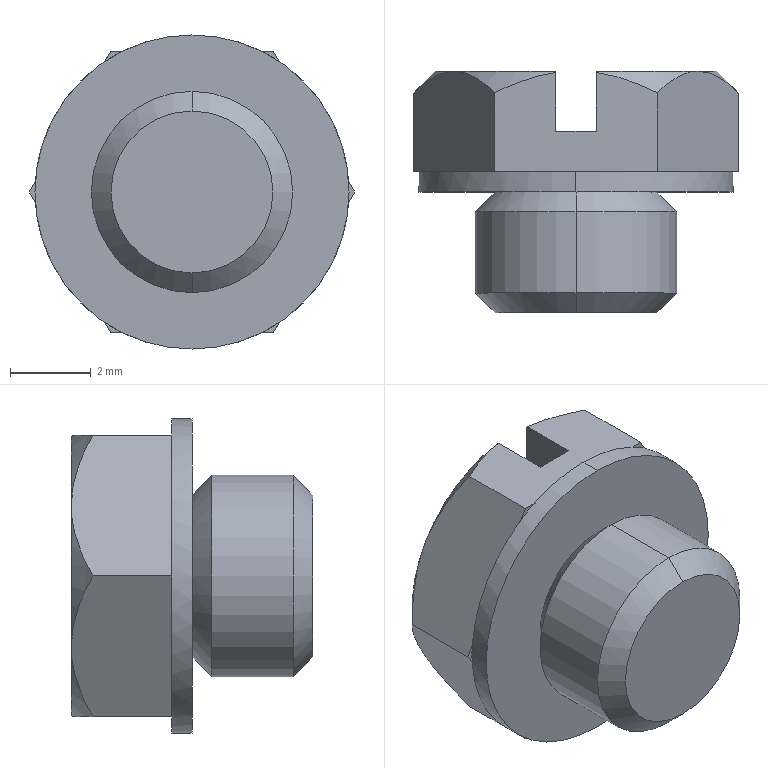Part | SolidWorks | features BaseBody 1 | 1 solid | 39 faces | box 8.083 x 6 x 7.8 mm | volume 174.211 mm3 | plane 25 | cone 10 | cylinder 4 | commonest cylinder face diameters 5 x2 7.8 x2
STEP:
#1=CARTESIAN_POINT('',(0.,-3.5,-2.01));
#2=VERTEX_POINT('',#1);
#3=CARTESIAN_POINT('',(0.,-3.5,2.01));
#4=VERTEX_POINT('',#3);
#5=CARTESIAN_POINT('',(0.,-3.5,0.));
#6=DIRECTION('',(0.,-1.,0.));
#7=DIRECTION('',(0.,0.,-1.));
#8=AXIS2_PLACEMENT_3D('',#5,#6,#7);
#9=CIRCLE('',#8,2.01);
#10=EDGE_CURVE('',#2,#4,#9,.T.);
#11=ORIENTED_EDGE('',*,*,#10,.F.);
#12=CARTESIAN_POINT('',(0.,-3.01,-2.5));
#13=VERTEX_POINT('',#12);
#14=CARTESIAN_POINT('',(0.,-3.01,-2.5));
#15=DIRECTION('',(0.,0.7071,-0.7071));
#16=VECTOR('',#15,1000.);
#17=LINE('',#14,#16);
#18=EDGE_CURVE('',#2,#13,#17,.T.);
#19=ORIENTED_EDGE('',*,*,#18,.T.);
#20=CARTESIAN_POINT('',(0.,-3.01,2.5));
#21=VERTEX_POINT('',#20);
#22=CARTESIAN_POINT('',(0.,-3.01,0.));
#23=DIRECTION('',(0.,-1.,0.));
#24=DIRECTION('',(0.,0.,-1.));
#25=AXIS2_PLACEMENT_3D('',#22,#23,#24);
#26=CIRCLE('',#25,2.5);
#27=EDGE_CURVE('',#13,#21,#26,.T.);
#28=ORIENTED_EDGE('',*,*,#27,.T.);
#29=CARTESIAN_POINT('',(0.,-3.01,2.5));
#30=DIRECTION('',(0.,0.7071,0.7071));
#31=VECTOR('',#30,1000.);
#32=LINE('',#29,#31);
#33=EDGE_CURVE('',#4,#21,#32,.T.);
#34=ORIENTED_EDGE('',*,*,#33,.F.);
#35=EDGE_LOOP('',(#11,#19,#28,#34));
#36=FACE_OUTER_BOUND('',#35,.T.);
#37=CARTESIAN_POINT('',(0.,-3.01,0.));
#38=DIRECTION('',(0.,1.,0.));
#39=DIRECTION('',(0.,0.,1.));
#40=AXIS2_PLACEMENT_3D('',#37,#38,#39);
#41=CONICAL_SURFACE('',#40,2.5,0.7854);
#42=ADVANCED_FACE('',(#36),#41,.T.);
#43=CARTESIAN_POINT('',(0.,-3.01,0.));
#44=DIRECTION('',(0.,-1.,0.));
#45=DIRECTION('',(0.,0.,-1.));
#46=AXIS2_PLACEMENT_3D('',#43,#44,#45);
#47=CIRCLE('',#46,2.5);
#48=EDGE_CURVE('',#21,#13,#47,.T.);
#49=ORIENTED_EDGE('',*,*,#48,.F.);
#50=CARTESIAN_POINT('',(0.,-0.9905,2.5));
#51=VERTEX_POINT('',#50);
#52=CARTESIAN_POINT('',(0.,-3.5,2.5));
#53=DIRECTION('',(0.,1.,0.));
#54=VECTOR('',#53,1000.);
#55=LINE('',#52,#54);
#56=EDGE_CURVE('',#21,#51,#55,.T.);
#57=ORIENTED_EDGE('',*,*,#56,.T.);
#58=CARTESIAN_POINT('',(0.,-0.9905,-2.5));
#59=VERTEX_POINT('',#58);
#60=CARTESIAN_POINT('',(0.,-0.9905,0.));
#61=DIRECTION('',(0.,-1.,0.));
#62=DIRECTION('',(0.,0.,-1.));
#63=AXIS2_PLACEMENT_3D('',#60,#61,#62);
#64=CIRCLE('',#63,2.5);
#65=EDGE_CURVE('',#51,#59,#64,.T.);
#66=ORIENTED_EDGE('',*,*,#65,.T.);
#67=CARTESIAN_POINT('',(0.,-3.5,-2.5));
#68=DIRECTION('',(0.,1.,0.));
#69=VECTOR('',#68,1000.);
#70=LINE('',#67,#69);
#71=EDGE_CURVE('',#13,#59,#70,.T.);
#72=ORIENTED_EDGE('',*,*,#71,.F.);
#73=EDGE_LOOP('',(#49,#57,#66,#72));
#74=FACE_OUTER_BOUND('',#73,.T.);
#75=CARTESIAN_POINT('',(0.,-3.5,0.));
#76=DIRECTION('',(0.,1.,0.));
#77=DIRECTION('',(0.,0.,-1.));
#78=AXIS2_PLACEMENT_3D('',#75,#76,#77);
#79=CYLINDRICAL_SURFACE('',#78,2.5);
#80=ADVANCED_FACE('',(#74),#79,.T.);
#81=CARTESIAN_POINT('',(0.,-0.5,-2.01));
#82=VERTEX_POINT('',#81);
#83=CARTESIAN_POINT('',(0.,-0.5,2.01));
#84=VERTEX_POINT('',#83);
#85=CARTESIAN_POINT('',(0.,-0.5,0.));
#86=DIRECTION('',(0.,-1.,0.));
#87=DIRECTION('',(0.,0.,-1.));
#88=AXIS2_PLACEMENT_3D('',#85,#86,#87);
#89=CIRCLE('',#88,2.01);
#90=EDGE_CURVE('',#82,#84,#89,.T.);
#91=ORIENTED_EDGE('',*,*,#90,.T.);
#92=CARTESIAN_POINT('',(0.,-0.5,2.01));
#93=DIRECTION('',(0.,-0.7071,0.7071));
#94=VECTOR('',#93,1000.);
#95=LINE('',#92,#94);
#96=EDGE_CURVE('',#84,#51,#95,.T.);
#97=ORIENTED_EDGE('',*,*,#96,.T.);
#98=CARTESIAN_POINT('',(0.,-0.9905,0.));
#99=DIRECTION('',(0.,-1.,0.));
#100=DIRECTION('',(0.,0.,-1.));
#101=AXIS2_PLACEMENT_3D('',#98,#99,#100);
#102=CIRCLE('',#101,2.5);
#103=EDGE_CURVE('',#59,#51,#102,.T.);
#104=ORIENTED_EDGE('',*,*,#103,.F.);
#105=CARTESIAN_POINT('',(0.,-0.5,-2.01));
#106=DIRECTION('',(0.,-0.7071,-0.7071));
#107=VECTOR('',#106,1000.);
#108=LINE('',#105,#107);
#109=EDGE_CURVE('',#82,#59,#108,.T.);
#110=ORIENTED_EDGE('',*,*,#109,.F.);
#111=EDGE_LOOP('',(#91,#97,#104,#110));
#112=FACE_OUTER_BOUND('',#111,.T.);
#113=CARTESIAN_POINT('',(0.,-0.5,0.));
#114=DIRECTION('',(0.,-1.,0.));
#115=DIRECTION('',(0.,0.,-1.));
#116=AXIS2_PLACEMENT_3D('',#113,#114,#115);
#117=CONICAL_SURFACE('',#116,2.01,0.7854);
#118=ADVANCED_FACE('',(#112),#117,.T.);
#119=CARTESIAN_POINT('',(0.,-0.5,3.9));
#120=VERTEX_POINT('',#119);
#121=CARTESIAN_POINT('',(0.,-0.5,-3.9));
#122=VERTEX_POINT('',#121);
#123=CARTESIAN_POINT('',(0.,-0.5,0.));
#124=DIRECTION('',(0.,-1.,0.));
#125=DIRECTION('',(0.,0.,-1.));
#126=AXIS2_PLACEMENT_3D('',#123,#124,#125);
#127=CIRCLE('',#126,3.9);
#128=EDGE_CURVE('',#120,#122,#127,.T.);
#129=ORIENTED_EDGE('',*,*,#128,.F.);
#130=CARTESIAN_POINT('',(0.,0.,3.9));
#131=VERTEX_POINT('',#130);
#132=CARTESIAN_POINT('',(0.,-0.5,3.9));
#133=DIRECTION('',(0.,1.,0.));
#134=VECTOR('',#133,1000.);
#135=LINE('',#132,#134);
#136=EDGE_CURVE('',#120,#131,#135,.T.);
#137=ORIENTED_EDGE('',*,*,#136,.T.);
#138=CARTESIAN_POINT('',(-1.72,0.,3.5));
#139=VERTEX_POINT('',#138);
#140=CARTESIAN_POINT('',(0.,0.,0.));
#141=DIRECTION('',(0.,-1.,0.));
#142=DIRECTION('',(0.,0.,-1.));
#143=AXIS2_PLACEMENT_3D('',#140,#141,#142);
#144=CIRCLE('',#143,3.9);
#145=EDGE_CURVE('',#131,#139,#144,.T.);
#146=ORIENTED_EDGE('',*,*,#145,.T.);
#147=CARTESIAN_POINT('',(-2.171,0.,3.24));
#148=VERTEX_POINT('',#147);
#149=CARTESIAN_POINT('',(0.,0.,0.));
#150=DIRECTION('',(0.,-1.,0.));
#151=DIRECTION('',(0.,0.,-1.));
#152=AXIS2_PLACEMENT_3D('',#149,#150,#151);
#153=CIRCLE('',#152,3.9);
#154=EDGE_CURVE('',#139,#148,#153,.T.);
#155=ORIENTED_EDGE('',*,*,#154,.T.);
#156=CARTESIAN_POINT('',(-3.891,0.,0.26));
#157=VERTEX_POINT('',#156);
#158=CARTESIAN_POINT('',(0.,0.,0.));
#159=DIRECTION('',(0.,-1.,0.));
#160=DIRECTION('',(0.,0.,-1.));
#161=AXIS2_PLACEMENT_3D('',#158,#159,#160);
#162=CIRCLE('',#161,3.9);
#163=EDGE_CURVE('',#148,#157,#162,.T.);
#164=ORIENTED_EDGE('',*,*,#163,.T.);
#165=CARTESIAN_POINT('',(-3.891,0.,-0.26));
#166=VERTEX_POINT('',#165);
#167=CARTESIAN_POINT('',(0.,0.,0.));
#168=DIRECTION('',(0.,-1.,0.));
#169=DIRECTION('',(0.,0.,-1.));
#170=AXIS2_PLACEMENT_3D('',#167,#168,#169);
#171=CIRCLE('',#170,3.9);
#172=EDGE_CURVE('',#157,#166,#171,.T.);
#173=ORIENTED_EDGE('',*,*,#172,.T.);
#174=CARTESIAN_POINT('',(-2.171,0.,-3.24));
#175=VERTEX_POINT('',#174);
#176=CARTESIAN_POINT('',(0.,0.,0.));
#177=DIRECTION('',(0.,-1.,0.));
#178=DIRECTION('',(0.,0.,-1.));
#179=AXIS2_PLACEMENT_3D('',#176,#177,#178);
#180=CIRCLE('',#179,3.9);
#181=EDGE_CURVE('',#166,#175,#180,.T.);
#182=ORIENTED_EDGE('',*,*,#181,.T.);
#183=CARTESIAN_POINT('',(-1.72,0.,-3.5));
#184=VERTEX_POINT('',#183);
#185=CARTESIAN_POINT('',(0.,0.,0.));
#186=DIRECTION('',(0.,-1.,0.));
#187=DIRECTION('',(0.,0.,-1.));
#188=AXIS2_PLACEMENT_3D('',#185,#186,#187);
#189=CIRCLE('',#188,3.9);
#190=EDGE_CURVE('',#175,#184,#189,.T.);
#191=ORIENTED_EDGE('',*,*,#190,.T.);
#192=CARTESIAN_POINT('',(0.,0.,-3.9));
#193=VERTEX_POINT('',#192);
#194=CARTESIAN_POINT('',(0.,0.,0.));
#195=DIRECTION('',(0.,-1.,0.));
#196=DIRECTION('',(0.,0.,-1.));
#197=AXIS2_PLACEMENT_3D('',#194,#195,#196);
#198=CIRCLE('',#197,3.9);
#199=EDGE_CURVE('',#184,#193,#198,.T.);
#200=ORIENTED_EDGE('',*,*,#199,.T.);
#201=CARTESIAN_POINT('',(0.,-0.5,-3.9));
#202=DIRECTION('',(0.,1.,0.));
#203=VECTOR('',#202,1000.);
#204=LINE('',#201,#203);
#205=EDGE_CURVE('',#122,#193,#204,.T.);
#206=ORIENTED_EDGE('',*,*,#205,.F.);
#207=EDGE_LOOP('',(#129,#137,#146,#155,#164,#173,#182,#191,#200,#206));
#208=FACE_OUTER_BOUND('',#207,.T.);
#209=CARTESIAN_POINT('',(0.,-0.5,0.));
#210=DIRECTION('',(0.,1.,0.));
#211=DIRECTION('',(0.,0.,-1.));
#212=AXIS2_PLACEMENT_3D('',#209,#210,#211);
#213=CYLINDRICAL_SURFACE('',#212,3.9);
#214=ADVANCED_FACE('',(#208),#213,.T.);
#215=CARTESIAN_POINT('',(-0.5,2.464,-3.5));
#216=VERTEX_POINT('',#215);
#217=CARTESIAN_POINT('',(-0.5,2.5,-3.464));
#218=VERTEX_POINT('',#217);
#219=CARTESIAN_POINT('',(-0.5,2.464,-3.5));
#220=CARTESIAN_POINT('',(-0.5,2.476,-3.488));
#221=CARTESIAN_POINT('',(-0.5,2.488,-3.476));
#222=CARTESIAN_POINT('',(-0.5,2.5,-3.464));
#223=B_SPLINE_CURVE_WITH_KNOTS('',3,(#219,#220,#221,#222),.UNSPECIFIED.,.F.,.F.,(4,4),(0.003913,0.003963),.UNSPECIFIED.);
#224=EDGE_CURVE('',#216,#218,#223,.T.);
#225=ORIENTED_EDGE('',*,*,#224,.F.);
#226=CARTESIAN_POINT('',(-2.021,1.959,-3.5));
#227=VERTEX_POINT('',#226);
#228=CARTESIAN_POINT('',(-0.5,2.464,-3.5));
#229=CARTESIAN_POINT('',(-0.6291,2.446,-3.5));
#230=CARTESIAN_POINT('',(-0.7576,2.421,-3.5));
#231=CARTESIAN_POINT('',(-0.9515,2.374,-3.5));
#232=CARTESIAN_POINT('',(-1.016,2.356,-3.5));
#233=CARTESIAN_POINT('',(-1.114,2.327,-3.5));
#234=CARTESIAN_POINT('',(-1.163,2.312,-3.5));
#235=CARTESIAN_POINT('',(-1.212,2.296,-3.5));
#236=CARTESIAN_POINT('',(-1.245,2.285,-3.5));
#237=CARTESIAN_POINT('',(-1.263,2.279,-3.5));
#238=CARTESIAN_POINT('',(-1.521,2.191,-3.5));
#239=CARTESIAN_POINT('',(-1.767,2.085,-3.5));
#240=CARTESIAN_POINT('',(-2.021,1.959,-3.5));
#241=B_SPLINE_CURVE_WITH_KNOTS('',3,(#228,#229,#230,#231,#232,#233,#234,#235,#236,#237,#238,#239,#240),.UNSPECIFIED.,.F.,.F.,(4,2,2,1,2,2,4),(0.,0.25,0.375,0.4375,0.4687,0.5,1.),.UNSPECIFIED.);
#242=EDGE_CURVE('',#216,#227,#241,.T.);
#243=ORIENTED_EDGE('',*,*,#242,.T.);
#244=CARTESIAN_POINT('',(-3.031,2.5,-1.75));
#245=VERTEX_POINT('',#244);
#246=CARTESIAN_POINT('',(-2.021,1.959,-3.5));
#247=CARTESIAN_POINT('',(-2.105,2.043,-3.354));
#248=CARTESIAN_POINT('',(-2.187,2.117,-3.212));
#249=CARTESIAN_POINT('',(-2.309,2.214,-3.001));
#250=CARTESIAN_POINT('',(-2.349,2.244,-2.932));
#251=CARTESIAN_POINT('',(-2.409,2.286,-2.827));
#252=CARTESIAN_POINT('',(-2.439,2.306,-2.775));
#253=CARTESIAN_POINT('',(-2.469,2.324,-2.723));
#254=CARTESIAN_POINT('',(-2.489,2.336,-2.689));
#255=CARTESIAN_POINT('',(-2.498,2.341,-2.673));
#256=CARTESIAN_POINT('',(-2.552,2.372,-2.58));
#257=CARTESIAN_POINT('',(-2.595,2.394,-2.505));
#258=CARTESIAN_POINT('',(-2.659,2.422,-2.394));
#259=CARTESIAN_POINT('',(-2.68,2.431,-2.358));
#260=CARTESIAN_POINT('',(-2.723,2.446,-2.284));
#261=CARTESIAN_POINT('',(-2.743,2.453,-2.248));
#262=CARTESIAN_POINT('',(-2.855,2.487,-2.056));
#263=CARTESIAN_POINT('',(-2.942,2.5,-1.904));
#264=CARTESIAN_POINT('',(-3.031,2.5,-1.75));
#265=B_SPLINE_CURVE_WITH_KNOTS('',3,(#246,#247,#248,#249,#250,#251,#252,#253,#254,#255,#256,#257,#258,#259,#260,#261,#262,#263,#264),.UNSPECIFIED.,.F.,.F.,(4,2,2,1,2,2,2,2,2,4),(0.,0.25,0.375,0.4375,0.4688,0.5,0.625,0.6875,0.75,1.),.UNSPECIFIED.);
#266=EDGE_CURVE('',#227,#245,#265,.T.);
#267=ORIENTED_EDGE('',*,*,#266,.T.);
#268=CARTESIAN_POINT('',(0.,2.5,0.));
#269=DIRECTION('',(0.,-1.,0.));
#270=DIRECTION('',(0.,0.,-1.));
#271=AXIS2_PLACEMENT_3D('',#268,#269,#270);
#272=CIRCLE('',#271,3.5);
#273=EDGE_CURVE('',#245,#218,#272,.T.);
#274=ORIENTED_EDGE('',*,*,#273,.T.);
#275=EDGE_LOOP('',(#225,#243,#267,#274));
#276=FACE_OUTER_BOUND('',#275,.T.);
#277=CARTESIAN_POINT('',(0.,2.5,0.));
#278=DIRECTION('',(0.,-1.,0.));
#279=DIRECTION('',(0.,0.,-1.));
#280=AXIS2_PLACEMENT_3D('',#277,#278,#279);
#281=CONICAL_SURFACE('',#280,3.5,0.7854);
#282=ADVANCED_FACE('',(#276),#281,.T.);
#283=CARTESIAN_POINT('',(-0.5,2.5,3.464));
#284=VERTEX_POINT('',#283);
#285=CARTESIAN_POINT('',(-0.5,2.464,3.5));
#286=VERTEX_POINT('',#285);
#287=CARTESIAN_POINT('',(-0.5,2.5,3.464));
#288=CARTESIAN_POINT('',(-0.5,2.488,3.476));
#289=CARTESIAN_POINT('',(-0.5,2.476,3.488));
#290=CARTESIAN_POINT('',(-0.5,2.464,3.5));
#291=B_SPLINE_CURVE_WITH_KNOTS('',3,(#287,#288,#289,#290),.UNSPECIFIED.,.F.,.F.,(4,4),(0.003847,0.003897),.UNSPECIFIED.);
#292=EDGE_CURVE('',#284,#286,#291,.T.);
#293=ORIENTED_EDGE('',*,*,#292,.T.);
#294=CARTESIAN_POINT('',(-0.5,1.,3.5));
#295=VERTEX_POINT('',#294);
#296=CARTESIAN_POINT('',(-0.5,5.,3.5));
#297=DIRECTION('',(0.,-1.,0.));
#298=VECTOR('',#297,1000.);
#299=LINE('',#296,#298);
#300=EDGE_CURVE('',#286,#295,#299,.T.);
#301=ORIENTED_EDGE('',*,*,#300,.T.);
#302=CARTESIAN_POINT('',(-0.5,1.,-3.5));
#303=VERTEX_POINT('',#302);
#304=CARTESIAN_POINT('',(-0.5,1.,5.));
#305=DIRECTION('',(0.,0.,-1.));
#306=VECTOR('',#305,1000.);
#307=LINE('',#304,#306);
#308=EDGE_CURVE('',#295,#303,#307,.T.);
#309=ORIENTED_EDGE('',*,*,#308,.T.);
#310=CARTESIAN_POINT('',(-0.5,5.,-3.5));
#311=DIRECTION('',(0.,1.,0.));
#312=VECTOR('',#311,1000.);
#313=LINE('',#310,#312);
#314=EDGE_CURVE('',#303,#216,#313,.T.);
#315=ORIENTED_EDGE('',*,*,#314,.T.);
#316=ORIENTED_EDGE('',*,*,#224,.T.);
#317=CARTESIAN_POINT('',(-0.5,2.5,5.));
#318=DIRECTION('',(0.,0.,-1.));
#319=VECTOR('',#318,1000.);
#320=LINE('',#317,#319);
#321=EDGE_CURVE('',#284,#218,#320,.T.);
#322=ORIENTED_EDGE('',*,*,#321,.F.);
#323=EDGE_LOOP('',(#293,#301,#309,#315,#316,#322));
#324=FACE_OUTER_BOUND('',#323,.T.);
#325=CARTESIAN_POINT('',(-0.5,2.5,5.));
#326=DIRECTION('',(1.,0.,0.));
#327=DIRECTION('',(0.,1.,0.));
#328=AXIS2_PLACEMENT_3D('',#325,#326,#327);
#329=PLANE('',#328);
#330=ADVANCED_FACE('',(#324),#329,.T.);
#331=CARTESIAN_POINT('',(2.171,0.,-3.24));
#332=VERTEX_POINT('',#331);
#333=CARTESIAN_POINT('',(3.891,0.,-0.26));
#334=VERTEX_POINT('',#333);
#335=CARTESIAN_POINT('',(0.,0.,0.));
#336=DIRECTION('',(0.,-1.,0.));
#337=DIRECTION('',(0.,0.,-1.));
#338=AXIS2_PLACEMENT_3D('',#335,#336,#337);
#339=CIRCLE('',#338,3.9);
#340=EDGE_CURVE('',#332,#334,#339,.T.);
#341=ORIENTED_EDGE('',*,*,#340,.F.);
#342=CARTESIAN_POINT('',(4.041,0.,0.));
#343=DIRECTION('',(0.5,0.,0.866));
#344=VECTOR('',#343,1000.);
#345=LINE('',#342,#344);
#346=EDGE_CURVE('',#332,#334,#345,.T.);
#347=ORIENTED_EDGE('',*,*,#346,.T.);
#348=EDGE_LOOP('',(#341,#347));
#349=FACE_OUTER_BOUND('',#348,.T.);
#350=CARTESIAN_POINT('',(0.,0.,0.));
#351=DIRECTION('',(0.,-1.,0.));
#352=DIRECTION('',(0.,0.,-1.));
#353=AXIS2_PLACEMENT_3D('',#350,#351,#352);
#354=PLANE('',#353);
#355=ADVANCED_FACE('',(#349),#354,.F.);
#356=CARTESIAN_POINT('',(3.891,0.,0.26));
#357=VERTEX_POINT('',#356);
#358=CARTESIAN_POINT('',(2.171,0.,3.24));
#359=VERTEX_POINT('',#358);
#360=CARTESIAN_POINT('',(0.,0.,0.));
#361=DIRECTION('',(0.,-1.,0.));
#362=DIRECTION('',(0.,0.,-1.));
#363=AXIS2_PLACEMENT_3D('',#360,#361,#362);
#364=CIRCLE('',#363,3.9);
#365=EDGE_CURVE('',#357,#359,#364,.T.);
#366=ORIENTED_EDGE('',*,*,#365,.F.);
#367=CARTESIAN_POINT('',(2.021,0.,3.5));
#368=DIRECTION('',(-0.5,0.,0.866));
#369=VECTOR('',#368,1000.);
#370=LINE('',#367,#369);
#371=EDGE_CURVE('',#357,#359,#370,.T.);
#372=ORIENTED_EDGE('',*,*,#371,.T.);
#373=EDGE_LOOP('',(#366,#372));
#374=FACE_OUTER_BOUND('',#373,.T.);
#375=CARTESIAN_POINT('',(0.,0.,0.));
#376=DIRECTION('',(0.,-1.,0.));
#377=DIRECTION('',(0.,0.,-1.));
#378=AXIS2_PLACEMENT_3D('',#375,#376,#377);
#379=PLANE('',#378);
#380=ADVANCED_FACE('',(#374),#379,.F.);
#381=ORIENTED_EDGE('',*,*,#199,.F.);
#382=CARTESIAN_POINT('',(1.72,0.,-3.5));
#383=VERTEX_POINT('',#382);
#384=CARTESIAN_POINT('',(2.021,0.,-3.5));
#385=DIRECTION('',(1.,0.,0.));
#386=VECTOR('',#385,1000.);
#387=LINE('',#384,#386);
#388=EDGE_CURVE('',#184,#383,#387,.T.);
#389=ORIENTED_EDGE('',*,*,#388,.T.);
#390=CARTESIAN_POINT('',(0.,0.,0.));
#391=DIRECTION('',(0.,-1.,0.));
#392=DIRECTION('',(0.,0.,-1.));
#393=AXIS2_PLACEMENT_3D('',#390,#391,#392);
#394=CIRCLE('',#393,3.9);
#395=EDGE_CURVE('',#193,#383,#394,.T.);
#396=ORIENTED_EDGE('',*,*,#395,.F.);
#397=EDGE_LOOP('',(#381,#389,#396));
#398=FACE_OUTER_BOUND('',#397,.T.);
#399=CARTESIAN_POINT('',(0.,0.,0.));
#400=DIRECTION('',(0.,-1.,0.));
#401=DIRECTION('',(0.,0.,-1.));
#402=AXIS2_PLACEMENT_3D('',#399,#400,#401);
#403=PLANE('',#402);
#404=ADVANCED_FACE('',(#398),#403,.F.);
#405=ORIENTED_EDGE('',*,*,#321,.T.);
#406=ORIENTED_EDGE('',*,*,#273,.F.);
#407=CARTESIAN_POINT('',(-3.031,2.5,1.75));
#408=VERTEX_POINT('',#407);
#409=CARTESIAN_POINT('',(0.,2.5,0.));
#410=DIRECTION('',(0.,-1.,0.));
#411=DIRECTION('',(0.,0.,-1.));
#412=AXIS2_PLACEMENT_3D('',#409,#410,#411);
#413=CIRCLE('',#412,3.5);
#414=EDGE_CURVE('',#408,#245,#413,.T.);
#415=ORIENTED_EDGE('',*,*,#414,.F.);
#416=CARTESIAN_POINT('',(0.,2.5,0.));
#417=DIRECTION('',(0.,-1.,0.));
#418=DIRECTION('',(0.,0.,-1.));
#419=AXIS2_PLACEMENT_3D('',#416,#417,#418);
#420=CIRCLE('',#419,3.5);
#421=EDGE_CURVE('',#284,#408,#420,.T.);
#422=ORIENTED_EDGE('',*,*,#421,.F.);
#423=EDGE_LOOP('',(#405,#406,#415,#422));
#424=FACE_OUTER_BOUND('',#423,.T.);
#425=CARTESIAN_POINT('',(0.,2.5,0.));
#426=DIRECTION('',(0.,-1.,0.));
#427=DIRECTION('',(0.,0.,-1.));
#428=AXIS2_PLACEMENT_3D('',#425,#426,#427);
#429=PLANE('',#428);
#430=ADVANCED_FACE('',(#424),#429,.F.);
#431=CARTESIAN_POINT('',(0.5,2.5,3.464));
#432=VERTEX_POINT('',#431);
#433=CARTESIAN_POINT('',(0.5,2.5,-3.464));
#434=VERTEX_POINT('',#433);
#435=CARTESIAN_POINT('',(0.5,2.5,5.));
#436=DIRECTION('',(0.,0.,-1.));
#437=VECTOR('',#436,1000.);
#438=LINE('',#435,#437);
#439=EDGE_CURVE('',#432,#434,#438,.T.);
#440=ORIENTED_EDGE('',*,*,#439,.F.);
#441=CARTESIAN_POINT('',(3.031,2.5,1.75));
#442=VERTEX_POINT('',#441);
#443=CARTESIAN_POINT('',(0.,2.5,0.));
#444=DIRECTION('',(0.,-1.,0.));
#445=DIRECTION('',(0.,0.,-1.));
#446=AXIS2_PLACEMENT_3D('',#443,#444,#445);
#447=CIRCLE('',#446,3.5);
#448=EDGE_CURVE('',#442,#432,#447,.T.);
#449=ORIENTED_EDGE('',*,*,#448,.F.);
#450=CARTESIAN_POINT('',(3.031,2.5,-1.75));
#451=VERTEX_POINT('',#450);
#452=CARTESIAN_POINT('',(0.,2.5,0.));
#453=DIRECTION('',(0.,-1.,0.));
#454=DIRECTION('',(0.,0.,-1.));
#455=AXIS2_PLACEMENT_3D('',#452,#453,#454);
#456=CIRCLE('',#455,3.5);
#457=EDGE_CURVE('',#451,#442,#456,.T.);
#458=ORIENTED_EDGE('',*,*,#457,.F.);
#459=CARTESIAN_POINT('',(0.,2.5,0.));
#460=DIRECTION('',(0.,-1.,0.));
#461=DIRECTION('',(0.,0.,-1.));
#462=AXIS2_PLACEMENT_3D('',#459,#460,#461);
#463=CIRCLE('',#462,3.5);
#464=EDGE_CURVE('',#434,#451,#463,.T.);
#465=ORIENTED_EDGE('',*,*,#464,.F.);
#466=EDGE_LOOP('',(#440,#449,#458,#465));
#467=FACE_OUTER_BOUND('',#466,.T.);
#468=CARTESIAN_POINT('',(0.,2.5,0.));
#469=DIRECTION('',(0.,-1.,0.));
#470=DIRECTION('',(0.,0.,-1.));
#471=AXIS2_PLACEMENT_3D('',#468,#469,#470);
#472=PLANE('',#471);
#473=ADVANCED_FACE('',(#467),#472,.F.);
#474=CARTESIAN_POINT('',(1.72,0.,3.5));
#475=VERTEX_POINT('',#474);
#476=CARTESIAN_POINT('',(0.,0.,0.));
#477=DIRECTION('',(0.,-1.,0.));
#478=DIRECTION('',(0.,0.,-1.));
#479=AXIS2_PLACEMENT_3D('',#476,#477,#478);
#480=CIRCLE('',#479,3.9);
#481=EDGE_CURVE('',#475,#131,#480,.T.);
#482=ORIENTED_EDGE('',*,*,#481,.F.);
#483=CARTESIAN_POINT('',(-2.021,0.,3.5));
#484=DIRECTION('',(-1.,0.,0.));
#485=VECTOR('',#484,1000.);
#486=LINE('',#483,#485);
#487=EDGE_CURVE('',#475,#139,#486,.T.);
#488=ORIENTED_EDGE('',*,*,#487,.T.);
#489=ORIENTED_EDGE('',*,*,#145,.F.);
#490=EDGE_LOOP('',(#482,#488,#489));
#491=FACE_OUTER_BOUND('',#490,.T.);
#492=CARTESIAN_POINT('',(0.,0.,0.));
#493=DIRECTION('',(0.,-1.,0.));
#494=DIRECTION('',(0.,0.,-1.));
#495=AXIS2_PLACEMENT_3D('',#492,#493,#494);
#496=PLANE('',#495);
#497=ADVANCED_FACE('',(#491),#496,.F.);
#498=ORIENTED_EDGE('',*,*,#163,.F.);
#499=CARTESIAN_POINT('',(-4.041,0.,0.));
#500=DIRECTION('',(0.5,0.,0.866));
#501=VECTOR('',#500,1000.);
#502=LINE('',#499,#501);
#503=EDGE_CURVE('',#157,#148,#502,.T.);
#504=ORIENTED_EDGE('',*,*,#503,.F.);
#505=EDGE_LOOP('',(#498,#504));
#506=FACE_OUTER_BOUND('',#505,.T.);
#507=CARTESIAN_POINT('',(0.,0.,0.));
#508=DIRECTION('',(0.,-1.,0.));
#509=DIRECTION('',(0.,0.,-1.));
#510=AXIS2_PLACEMENT_3D('',#507,#508,#509);
#511=PLANE('',#510);
#512=ADVANCED_FACE('',(#506),#511,.F.);
#513=ORIENTED_EDGE('',*,*,#136,.F.);
#514=CARTESIAN_POINT('',(0.,-0.5,0.));
#515=DIRECTION('',(0.,-1.,0.));
#516=DIRECTION('',(0.,0.,-1.));
#517=AXIS2_PLACEMENT_3D('',#514,#515,#516);
#518=CIRCLE('',#517,3.9);
#519=EDGE_CURVE('',#122,#120,#518,.T.);
#520=ORIENTED_EDGE('',*,*,#519,.F.);
#521=ORIENTED_EDGE('',*,*,#205,.T.);
#522=ORIENTED_EDGE('',*,*,#395,.T.);
#523=CARTESIAN_POINT('',(0.,0.,0.));
#524=DIRECTION('',(0.,-1.,0.));
#525=DIRECTION('',(0.,0.,-1.));
#526=AXIS2_PLACEMENT_3D('',#523,#524,#525);
#527=CIRCLE('',#526,3.9);
#528=EDGE_CURVE('',#383,#332,#527,.T.);
#529=ORIENTED_EDGE('',*,*,#528,.T.);
#530=ORIENTED_EDGE('',*,*,#340,.T.);
#531=CARTESIAN_POINT('',(0.,0.,0.));
#532=DIRECTION('',(0.,-1.,0.));
#533=DIRECTION('',(0.,0.,-1.));
#534=AXIS2_PLACEMENT_3D('',#531,#532,#533);
#535=CIRCLE('',#534,3.9);
#536=EDGE_CURVE('',#334,#357,#535,.T.);
#537=ORIENTED_EDGE('',*,*,#536,.T.);
#538=ORIENTED_EDGE('',*,*,#365,.T.);
#539=CARTESIAN_POINT('',(0.,0.,0.));
#540=DIRECTION('',(0.,-1.,0.));
#541=DIRECTION('',(0.,0.,-1.));
#542=AXIS2_PLACEMENT_3D('',#539,#540,#541);
#543=CIRCLE('',#542,3.9);
#544=EDGE_CURVE('',#359,#475,#543,.T.);
#545=ORIENTED_EDGE('',*,*,#544,.T.);
#546=ORIENTED_EDGE('',*,*,#481,.T.);
#547=EDGE_LOOP('',(#513,#520,#521,#522,#529,#530,#537,#538,#545,#546));
#548=FACE_OUTER_BOUND('',#547,.T.);
#549=CARTESIAN_POINT('',(0.,-0.5,0.));
#550=DIRECTION('',(0.,1.,0.));
#551=DIRECTION('',(0.,0.,-1.));
#552=AXIS2_PLACEMENT_3D('',#549,#550,#551);
#553=CYLINDRICAL_SURFACE('',#552,3.9);
#554=ADVANCED_FACE('',(#548),#553,.T.);
#555=ORIENTED_EDGE('',*,*,#181,.F.);
#556=CARTESIAN_POINT('',(-2.021,0.,-3.5));
#557=DIRECTION('',(0.5,0.,-0.866));
#558=VECTOR('',#557,1000.);
#559=LINE('',#556,#558);
#560=EDGE_CURVE('',#166,#175,#559,.T.);
#561=ORIENTED_EDGE('',*,*,#560,.T.);
#562=EDGE_LOOP('',(#555,#561));
#563=FACE_OUTER_BOUND('',#562,.T.);
#564=CARTESIAN_POINT('',(0.,0.,0.));
#565=DIRECTION('',(0.,-1.,0.));
#566=DIRECTION('',(0.,0.,-1.));
#567=AXIS2_PLACEMENT_3D('',#564,#565,#566);
#568=PLANE('',#567);
#569=ADVANCED_FACE('',(#563),#568,.F.);
#570=CARTESIAN_POINT('',(0.,-3.5,0.));
#571=DIRECTION('',(0.,-1.,0.));
#572=DIRECTION('',(0.,0.,-1.));
#573=AXIS2_PLACEMENT_3D('',#570,#571,#572);
#574=CIRCLE('',#573,2.01);
#575=EDGE_CURVE('',#4,#2,#574,.T.);
#576=ORIENTED_EDGE('',*,*,#575,.T.);
#577=ORIENTED_EDGE('',*,*,#10,.T.);
#578=EDGE_LOOP('',(#576,#577));
#579=FACE_OUTER_BOUND('',#578,.T.);
#580=CARTESIAN_POINT('',(2.01,-3.5,0.));
#581=DIRECTION('',(0.,1.,0.));
#582=DIRECTION('',(1.,0.,0.));
#583=AXIS2_PLACEMENT_3D('',#580,#581,#582);
#584=PLANE('',#583);
#585=ADVANCED_FACE('',(#579),#584,.F.);
#586=CARTESIAN_POINT('',(0.5,2.464,-3.5));
#587=VERTEX_POINT('',#586);
#588=CARTESIAN_POINT('',(0.5,2.5,-3.464));
#589=CARTESIAN_POINT('',(0.5,2.488,-3.476));
#590=CARTESIAN_POINT('',(0.5,2.476,-3.488));
#591=CARTESIAN_POINT('',(0.5,2.464,-3.5));
#592=B_SPLINE_CURVE_WITH_KNOTS('',3,(#588,#589,#590,#591),.UNSPECIFIED.,.F.,.F.,(4,4),(0.003823,0.003873),.UNSPECIFIED.);
#593=EDGE_CURVE('',#434,#587,#592,.T.);
#594=ORIENTED_EDGE('',*,*,#593,.F.);
#595=ORIENTED_EDGE('',*,*,#464,.T.);
#596=CARTESIAN_POINT('',(2.021,1.959,-3.5));
#597=VERTEX_POINT('',#596);
#598=CARTESIAN_POINT('',(3.031,2.5,-1.75));
#599=CARTESIAN_POINT('',(2.988,2.5,-1.825));
#600=CARTESIAN_POINT('',(2.944,2.497,-1.901));
#601=CARTESIAN_POINT('',(2.857,2.484,-2.051));
#602=CARTESIAN_POINT('',(2.813,2.474,-2.129));
#603=CARTESIAN_POINT('',(2.727,2.448,-2.277));
#604=CARTESIAN_POINT('',(2.684,2.433,-2.351));
#605=CARTESIAN_POINT('',(2.62,2.405,-2.462));
#606=CARTESIAN_POINT('',(2.588,2.39,-2.518));
#607=CARTESIAN_POINT('',(2.555,2.373,-2.574));
#608=CARTESIAN_POINT('',(2.534,2.362,-2.611));
#609=CARTESIAN_POINT('',(2.522,2.355,-2.631));
#610=CARTESIAN_POINT('',(2.352,2.258,-2.927));
#611=CARTESIAN_POINT('',(2.19,2.128,-3.207));
#612=CARTESIAN_POINT('',(2.021,1.959,-3.5));
#613=B_SPLINE_CURVE_WITH_KNOTS('',3,(#598,#599,#600,#601,#602,#603,#604,#605,#606,#607,#608,#609,#610,#611,#612),.UNSPECIFIED.,.F.,.F.,(4,2,2,2,1,2,2,4),(0.,0.125,0.25,0.375,0.4375,0.4687,0.5,1.),.UNSPECIFIED.);
#614=EDGE_CURVE('',#451,#597,#613,.T.);
#615=ORIENTED_EDGE('',*,*,#614,.T.);
#616=CARTESIAN_POINT('',(2.021,1.959,-3.5));
#617=CARTESIAN_POINT('',(1.894,2.022,-3.5));
#618=CARTESIAN_POINT('',(1.77,2.08,-3.5));
#619=CARTESIAN_POINT('',(1.585,2.158,-3.5));
#620=CARTESIAN_POINT('',(1.493,2.196,-3.5));
#621=CARTESIAN_POINT('',(1.386,2.236,-3.5));
#622=CARTESIAN_POINT('',(1.341,2.252,-3.5));
#623=CARTESIAN_POINT('',(1.31,2.263,-3.5));
#624=CARTESIAN_POINT('',(1.297,2.268,-3.5));
#625=CARTESIAN_POINT('',(1.016,2.364,-3.5));
#626=CARTESIAN_POINT('',(0.759,2.428,-3.5));
#627=CARTESIAN_POINT('',(0.5,2.464,-3.5));
#628=B_SPLINE_CURVE_WITH_KNOTS('',3,(#616,#617,#618,#619,#620,#621,#622,#623,#624,#625,#626,#627),.UNSPECIFIED.,.F.,.F.,(4,2,1,1,2,2,4),(0.,0.25,0.375,0.4375,0.4687,0.5,1.),.UNSPECIFIED.);
#629=EDGE_CURVE('',#597,#587,#628,.T.);
#630=ORIENTED_EDGE('',*,*,#629,.T.);
#631=EDGE_LOOP('',(#594,#595,#615,#630));
#632=FACE_OUTER_BOUND('',#631,.T.);
#633=CARTESIAN_POINT('',(0.,2.5,0.));
#634=DIRECTION('',(0.,-1.,0.));
#635=DIRECTION('',(0.,0.,-1.));
#636=AXIS2_PLACEMENT_3D('',#633,#634,#635);
#637=CONICAL_SURFACE('',#636,3.5,0.7854);
#638=ADVANCED_FACE('',(#632),#637,.T.);
#639=CARTESIAN_POINT('',(0.5,2.464,3.5));
#640=VERTEX_POINT('',#639);
#641=CARTESIAN_POINT('',(0.5,2.464,3.5));
#642=CARTESIAN_POINT('',(0.5,2.476,3.488));
#643=CARTESIAN_POINT('',(0.5,2.488,3.476));
#644=CARTESIAN_POINT('',(0.5,2.5,3.464));
#645=B_SPLINE_CURVE_WITH_KNOTS('',3,(#641,#642,#643,#644),.UNSPECIFIED.,.F.,.F.,(4,4),(0.003913,0.003963),.UNSPECIFIED.);
#646=EDGE_CURVE('',#640,#432,#645,.T.);
#647=ORIENTED_EDGE('',*,*,#646,.F.);
#648=CARTESIAN_POINT('',(2.021,1.959,3.5));
#649=VERTEX_POINT('',#648);
#650=CARTESIAN_POINT('',(0.5,2.464,3.5));
#651=CARTESIAN_POINT('',(0.6295,2.446,3.5));
#652=CARTESIAN_POINT('',(0.7583,2.421,3.5));
#653=CARTESIAN_POINT('',(0.9527,2.373,3.5));
#654=CARTESIAN_POINT('',(1.018,2.356,3.5));
#655=CARTESIAN_POINT('',(1.116,2.327,3.5));
#656=CARTESIAN_POINT('',(1.165,2.311,3.5));
#657=CARTESIAN_POINT('',(1.214,2.295,3.5));
#658=CARTESIAN_POINT('',(1.247,2.284,3.5));
#659=CARTESIAN_POINT('',(1.265,2.278,3.5));
#660=CARTESIAN_POINT('',(1.522,2.19,3.5));
#661=CARTESIAN_POINT('',(1.768,2.085,3.5));
#662=CARTESIAN_POINT('',(2.021,1.959,3.5));
#663=B_SPLINE_CURVE_WITH_KNOTS('',3,(#650,#651,#652,#653,#654,#655,#656,#657,#658,#659,#660,#661,#662),.UNSPECIFIED.,.F.,.F.,(4,2,2,1,2,2,4),(0.,0.25,0.375,0.4375,0.4687,0.5,1.),.UNSPECIFIED.);
#664=EDGE_CURVE('',#640,#649,#663,.T.);
#665=ORIENTED_EDGE('',*,*,#664,.T.);
#666=CARTESIAN_POINT('',(2.021,1.959,3.5));
#667=CARTESIAN_POINT('',(2.105,2.043,3.354));
#668=CARTESIAN_POINT('',(2.187,2.117,3.212));
#669=CARTESIAN_POINT('',(2.309,2.214,3.001));
#670=CARTESIAN_POINT('',(2.349,2.244,2.932));
#671=CARTESIAN_POINT('',(2.409,2.286,2.827));
#672=CARTESIAN_POINT('',(2.439,2.306,2.775));
#673=CARTESIAN_POINT('',(2.469,2.324,2.723));
#674=CARTESIAN_POINT('',(2.489,2.336,2.689));
#675=CARTESIAN_POINT('',(2.498,2.341,2.673));
#676=CARTESIAN_POINT('',(2.552,2.372,2.58));
#677=CARTESIAN_POINT('',(2.595,2.394,2.505));
#678=CARTESIAN_POINT('',(2.659,2.422,2.394));
#679=CARTESIAN_POINT('',(2.68,2.431,2.358));
#680=CARTESIAN_POINT('',(2.723,2.446,2.284));
#681=CARTESIAN_POINT('',(2.743,2.453,2.248));
#682=CARTESIAN_POINT('',(2.855,2.487,2.056));
#683=CARTESIAN_POINT('',(2.942,2.5,1.904));
#684=CARTESIAN_POINT('',(3.031,2.5,1.75));
#685=B_SPLINE_CURVE_WITH_KNOTS('',3,(#666,#667,#668,#669,#670,#671,#672,#673,#674,#675,#676,#677,#678,#679,#680,#681,#682,#683,#684),.UNSPECIFIED.,.F.,.F.,(4,2,2,1,2,2,2,2,2,4),(0.,0.25,0.375,0.4375,0.4687,0.5,0.625,0.6875,0.75,1.),.UNSPECIFIED.);
#686=EDGE_CURVE('',#649,#442,#685,.T.);
#687=ORIENTED_EDGE('',*,*,#686,.T.);
#688=ORIENTED_EDGE('',*,*,#448,.T.);
#689=EDGE_LOOP('',(#647,#665,#687,#688));
#690=FACE_OUTER_BOUND('',#689,.T.);
#691=CARTESIAN_POINT('',(0.,2.5,0.));
#692=DIRECTION('',(0.,-1.,0.));
#693=DIRECTION('',(0.,0.,-1.));
#694=AXIS2_PLACEMENT_3D('',#691,#692,#693);
#695=CONICAL_SURFACE('',#694,3.5,0.7854);
#696=ADVANCED_FACE('',(#690),#695,.T.);
#697=ORIENTED_EDGE('',*,*,#292,.F.);
#698=ORIENTED_EDGE('',*,*,#421,.T.);
#699=CARTESIAN_POINT('',(-2.021,1.959,3.5));
#700=VERTEX_POINT('',#699);
#701=CARTESIAN_POINT('',(-3.031,2.5,1.75));
#702=CARTESIAN_POINT('',(-2.988,2.5,1.825));
#703=CARTESIAN_POINT('',(-2.944,2.497,1.901));
#704=CARTESIAN_POINT('',(-2.857,2.484,2.051));
#705=CARTESIAN_POINT('',(-2.813,2.474,2.129));
#706=CARTESIAN_POINT('',(-2.727,2.448,2.277));
#707=CARTESIAN_POINT('',(-2.684,2.433,2.351));
#708=CARTESIAN_POINT('',(-2.62,2.405,2.462));
#709=CARTESIAN_POINT('',(-2.588,2.39,2.518));
#710=CARTESIAN_POINT('',(-2.555,2.373,2.574));
#711=CARTESIAN_POINT('',(-2.534,2.362,2.611));
#712=CARTESIAN_POINT('',(-2.522,2.355,2.631));
#713=CARTESIAN_POINT('',(-2.352,2.258,2.927));
#714=CARTESIAN_POINT('',(-2.19,2.128,3.207));
#715=CARTESIAN_POINT('',(-2.021,1.959,3.5));
#716=B_SPLINE_CURVE_WITH_KNOTS('',3,(#701,#702,#703,#704,#705,#706,#707,#708,#709,#710,#711,#712,#713,#714,#715),.UNSPECIFIED.,.F.,.F.,(4,2,2,2,1,2,2,4),(0.,0.125,0.25,0.375,0.4375,0.4687,0.5,1.),.UNSPECIFIED.);
#717=EDGE_CURVE('',#408,#700,#716,.T.);
#718=ORIENTED_EDGE('',*,*,#717,.T.);
#719=CARTESIAN_POINT('',(-2.021,1.959,3.5));
#720=CARTESIAN_POINT('',(-1.894,2.022,3.5));
#721=CARTESIAN_POINT('',(-1.769,2.08,3.5));
#722=CARTESIAN_POINT('',(-1.584,2.159,3.5));
#723=CARTESIAN_POINT('',(-1.491,2.196,3.5));
#724=CARTESIAN_POINT('',(-1.385,2.236,3.5));
#725=CARTESIAN_POINT('',(-1.339,2.253,3.5));
#726=CARTESIAN_POINT('',(-1.308,2.263,3.5));
#727=CARTESIAN_POINT('',(-1.295,2.268,3.5));
#728=CARTESIAN_POINT('',(-1.014,2.364,3.5));
#729=CARTESIAN_POINT('',(-0.7583,2.428,3.5));
#730=CARTESIAN_POINT('',(-0.5,2.464,3.5));
#731=B_SPLINE_CURVE_WITH_KNOTS('',3,(#719,#720,#721,#722,#723,#724,#725,#726,#727,#728,#729,#730),.UNSPECIFIED.,.F.,.F.,(4,2,1,1,2,2,4),(0.,0.25,0.375,0.4375,0.4688,0.5,1.),.UNSPECIFIED.);
#732=EDGE_CURVE('',#700,#286,#731,.T.);
#733=ORIENTED_EDGE('',*,*,#732,.T.);
#734=EDGE_LOOP('',(#697,#698,#718,#733));
#735=FACE_OUTER_BOUND('',#734,.T.);
#736=CARTESIAN_POINT('',(0.,2.5,0.));
#737=DIRECTION('',(0.,-1.,0.));
#738=DIRECTION('',(0.,0.,-1.));
#739=AXIS2_PLACEMENT_3D('',#736,#737,#738);
#740=CONICAL_SURFACE('',#739,3.5,0.7854);
#741=ADVANCED_FACE('',(#735),#740,.T.);
#742=ORIENTED_EDGE('',*,*,#300,.F.);
#743=ORIENTED_EDGE('',*,*,#732,.F.);
#744=CARTESIAN_POINT('',(-2.021,0.,3.5));
#745=VERTEX_POINT('',#744);
#746=CARTESIAN_POINT('',(-2.021,5.,3.5));
#747=DIRECTION('',(0.,-1.,0.));
#748=VECTOR('',#747,1000.);
#749=LINE('',#746,#748);
#750=EDGE_CURVE('',#700,#745,#749,.T.);
#751=ORIENTED_EDGE('',*,*,#750,.T.);
#752=CARTESIAN_POINT('',(-2.021,0.,3.5));
#753=DIRECTION('',(1.,0.,0.));
#754=VECTOR('',#753,1000.);
#755=LINE('',#752,#754);
#756=EDGE_CURVE('',#745,#139,#755,.T.);
#757=ORIENTED_EDGE('',*,*,#756,.T.);
#758=ORIENTED_EDGE('',*,*,#487,.F.);
#759=CARTESIAN_POINT('',(2.021,0.,3.5));
#760=VERTEX_POINT('',#759);
#761=CARTESIAN_POINT('',(-2.021,0.,3.5));
#762=DIRECTION('',(1.,0.,0.));
#763=VECTOR('',#762,1000.);
#764=LINE('',#761,#763);
#765=EDGE_CURVE('',#475,#760,#764,.T.);
#766=ORIENTED_EDGE('',*,*,#765,.T.);
#767=CARTESIAN_POINT('',(2.021,5.,3.5));
#768=DIRECTION('',(0.,-1.,0.));
#769=VECTOR('',#768,1000.);
#770=LINE('',#767,#769);
#771=EDGE_CURVE('',#649,#760,#770,.T.);
#772=ORIENTED_EDGE('',*,*,#771,.F.);
#773=ORIENTED_EDGE('',*,*,#664,.F.);
#774=CARTESIAN_POINT('',(0.5,1.,3.5));
#775=VERTEX_POINT('',#774);
#776=CARTESIAN_POINT('',(0.5,5.,3.5));
#777=DIRECTION('',(0.,1.,0.));
#778=VECTOR('',#777,1000.);
#779=LINE('',#776,#778);
#780=EDGE_CURVE('',#775,#640,#779,.T.);
#781=ORIENTED_EDGE('',*,*,#780,.F.);
#782=CARTESIAN_POINT('',(-2.021,1.,3.5));
#783=DIRECTION('',(1.,0.,0.));
#784=VECTOR('',#783,1000.);
#785=LINE('',#782,#784);
#786=EDGE_CURVE('',#295,#775,#785,.T.);
#787=ORIENTED_EDGE('',*,*,#786,.F.);
#788=EDGE_LOOP('',(#742,#743,#751,#757,#758,#766,#772,#773,#781,#787));
#789=FACE_OUTER_BOUND('',#788,.T.);
#790=CARTESIAN_POINT('',(-2.021,5.,3.5));
#791=DIRECTION('',(0.,0.,-1.));
#792=DIRECTION('',(0.,-1.,0.));
#793=AXIS2_PLACEMENT_3D('',#790,#791,#792);
#794=PLANE('',#793);
#795=ADVANCED_FACE('',(#789),#794,.F.);
#796=ORIENTED_EDGE('',*,*,#457,.T.);
#797=CARTESIAN_POINT('',(4.041,1.959,0.));
#798=VERTEX_POINT('',#797);
#799=CARTESIAN_POINT('',(3.031,2.5,1.75));
#800=CARTESIAN_POINT('',(3.075,2.5,1.675));
#801=CARTESIAN_POINT('',(3.118,2.497,1.599));
#802=CARTESIAN_POINT('',(3.205,2.484,1.449));
#803=CARTESIAN_POINT('',(3.25,2.474,1.371));
#804=CARTESIAN_POINT('',(3.335,2.448,1.223));
#805=CARTESIAN_POINT('',(3.378,2.433,1.149));
#806=CARTESIAN_POINT('',(3.442,2.405,1.038));
#807=CARTESIAN_POINT('',(3.475,2.39,0.982));
#808=CARTESIAN_POINT('',(3.507,2.373,0.926));
#809=CARTESIAN_POINT('',(3.528,2.362,0.8887));
#810=CARTESIAN_POINT('',(3.54,2.355,0.8687));
#811=CARTESIAN_POINT('',(3.711,2.258,0.5731));
#812=CARTESIAN_POINT('',(3.872,2.128,0.2932));
#813=CARTESIAN_POINT('',(4.041,1.959,0.));
#814=B_SPLINE_CURVE_WITH_KNOTS('',3,(#799,#800,#801,#802,#803,#804,#805,#806,#807,#808,#809,#810,#811,#812,#813),.UNSPECIFIED.,.F.,.F.,(4,2,2,2,1,2,2,4),(0.,0.125,0.25,0.375,0.4375,0.4688,0.5,1.),.UNSPECIFIED.);
#815=EDGE_CURVE('',#442,#798,#814,.T.);
#816=ORIENTED_EDGE('',*,*,#815,.T.);
#817=CARTESIAN_POINT('',(4.041,1.959,0.));
#818=CARTESIAN_POINT('',(3.957,2.043,-0.1456));
#819=CARTESIAN_POINT('',(3.875,2.117,-0.2879));
#820=CARTESIAN_POINT('',(3.753,2.214,-0.4987));
#821=CARTESIAN_POINT('',(3.713,2.244,-0.5684));
#822=CARTESIAN_POINT('',(3.653,2.286,-0.6727));
#823=CARTESIAN_POINT('',(3.623,2.306,-0.7247));
#824=CARTESIAN_POINT('',(3.593,2.324,-0.7766));
#825=CARTESIAN_POINT('',(3.573,2.336,-0.8111));
#826=CARTESIAN_POINT('',(3.564,2.341,-0.827));
#827=CARTESIAN_POINT('',(3.51,2.372,-0.9204));
#828=CARTESIAN_POINT('',(3.467,2.394,-0.9946));
#829=CARTESIAN_POINT('',(3.403,2.422,-1.106));
#830=CARTESIAN_POINT('',(3.382,2.431,-1.142));
#831=CARTESIAN_POINT('',(3.339,2.446,-1.216));
#832=CARTESIAN_POINT('',(3.319,2.453,-1.252));
#833=CARTESIAN_POINT('',(3.208,2.487,-1.444));
#834=CARTESIAN_POINT('',(3.12,2.5,-1.596));
#835=CARTESIAN_POINT('',(3.031,2.5,-1.75));
#836=B_SPLINE_CURVE_WITH_KNOTS('',3,(#817,#818,#819,#820,#821,#822,#823,#824,#825,#826,#827,#828,#829,#830,#831,#832,#833,#834,#835),.UNSPECIFIED.,.F.,.F.,(4,2,2,1,2,2,2,2,2,4),(0.,0.25,0.375,0.4375,0.4687,0.5,0.625,0.6875,0.75,1.),.UNSPECIFIED.);
#837=EDGE_CURVE('',#798,#451,#836,.T.);
#838=ORIENTED_EDGE('',*,*,#837,.T.);
#839=EDGE_LOOP('',(#796,#816,#838));
#840=FACE_OUTER_BOUND('',#839,.T.);
#841=CARTESIAN_POINT('',(0.,2.5,0.));
#842=DIRECTION('',(0.,-1.,0.));
#843=DIRECTION('',(0.,0.,-1.));
#844=AXIS2_PLACEMENT_3D('',#841,#842,#843);
#845=CONICAL_SURFACE('',#844,3.5,0.7854);
#846=ADVANCED_FACE('',(#840),#845,.T.);
#847=ORIENTED_EDGE('',*,*,#414,.T.);
#848=CARTESIAN_POINT('',(-4.041,1.959,0.));
#849=VERTEX_POINT('',#848);
#850=CARTESIAN_POINT('',(-3.031,2.5,-1.75));
#851=CARTESIAN_POINT('',(-3.075,2.5,-1.675));
#852=CARTESIAN_POINT('',(-3.118,2.497,-1.599));
#853=CARTESIAN_POINT('',(-3.205,2.484,-1.449));
#854=CARTESIAN_POINT('',(-3.25,2.474,-1.371));
#855=CARTESIAN_POINT('',(-3.335,2.448,-1.223));
#856=CARTESIAN_POINT('',(-3.378,2.433,-1.149));
#857=CARTESIAN_POINT('',(-3.442,2.405,-1.038));
#858=CARTESIAN_POINT('',(-3.475,2.39,-0.982));
#859=CARTESIAN_POINT('',(-3.507,2.373,-0.926));
#860=CARTESIAN_POINT('',(-3.528,2.362,-0.8887));
#861=CARTESIAN_POINT('',(-3.54,2.355,-0.8687));
#862=CARTESIAN_POINT('',(-3.711,2.258,-0.5731));
#863=CARTESIAN_POINT('',(-3.872,2.128,-0.2932));
#864=CARTESIAN_POINT('',(-4.041,1.959,0.));
#865=B_SPLINE_CURVE_WITH_KNOTS('',3,(#850,#851,#852,#853,#854,#855,#856,#857,#858,#859,#860,#861,#862,#863,#864),.UNSPECIFIED.,.F.,.F.,(4,2,2,2,1,2,2,4),(0.,0.125,0.25,0.375,0.4375,0.4687,0.5,1.),.UNSPECIFIED.);
#866=EDGE_CURVE('',#245,#849,#865,.T.);
#867=ORIENTED_EDGE('',*,*,#866,.T.);
#868=CARTESIAN_POINT('',(-4.041,1.959,0.));
#869=CARTESIAN_POINT('',(-3.957,2.043,0.1456));
#870=CARTESIAN_POINT('',(-3.875,2.117,0.2879));
#871=CARTESIAN_POINT('',(-3.753,2.214,0.4987));
#872=CARTESIAN_POINT('',(-3.713,2.244,0.5684));
#873=CARTESIAN_POINT('',(-3.653,2.286,0.6727));
#874=CARTESIAN_POINT('',(-3.623,2.306,0.7247));
#875=CARTESIAN_POINT('',(-3.593,2.324,0.7766));
#876=CARTESIAN_POINT('',(-3.573,2.336,0.8111));
#877=CARTESIAN_POINT('',(-3.564,2.341,0.827));
#878=CARTESIAN_POINT('',(-3.51,2.372,0.9204));
#879=CARTESIAN_POINT('',(-3.467,2.394,0.9946));
#880=CARTESIAN_POINT('',(-3.403,2.422,1.106));
#881=CARTESIAN_POINT('',(-3.382,2.431,1.142));
#882=CARTESIAN_POINT('',(-3.339,2.446,1.216));
#883=CARTESIAN_POINT('',(-3.319,2.453,1.252));
#884=CARTESIAN_POINT('',(-3.208,2.487,1.444));
#885=CARTESIAN_POINT('',(-3.12,2.5,1.596));
#886=CARTESIAN_POINT('',(-3.031,2.5,1.75));
#887=B_SPLINE_CURVE_WITH_KNOTS('',3,(#868,#869,#870,#871,#872,#873,#874,#875,#876,#877,#878,#879,#880,#881,#882,#883,#884,#885,#886),.UNSPECIFIED.,.F.,.F.,(4,2,2,1,2,2,2,2,2,4),(0.,0.25,0.375,0.4375,0.4687,0.5,0.625,0.6875,0.75,1.),.UNSPECIFIED.);
#888=EDGE_CURVE('',#849,#408,#887,.T.);
#889=ORIENTED_EDGE('',*,*,#888,.T.);
#890=EDGE_LOOP('',(#847,#867,#889));
#891=FACE_OUTER_BOUND('',#890,.T.);
#892=CARTESIAN_POINT('',(0.,2.5,0.));
#893=DIRECTION('',(0.,-1.,0.));
#894=DIRECTION('',(0.,0.,-1.));
#895=AXIS2_PLACEMENT_3D('',#892,#893,#894);
#896=CONICAL_SURFACE('',#895,3.5,0.7854);
#897=ADVANCED_FACE('',(#891),#896,.T.);
#898=ORIENTED_EDGE('',*,*,#519,.T.);
#899=ORIENTED_EDGE('',*,*,#128,.T.);
#900=EDGE_LOOP('',(#898,#899));
#901=FACE_OUTER_BOUND('',#900,.T.);
#902=ORIENTED_EDGE('',*,*,#90,.F.);
#903=CARTESIAN_POINT('',(0.,-0.5,0.));
#904=DIRECTION('',(0.,-1.,0.));
#905=DIRECTION('',(0.,0.,-1.));
#906=AXIS2_PLACEMENT_3D('',#903,#904,#905);
#907=CIRCLE('',#906,2.01);
#908=EDGE_CURVE('',#84,#82,#907,.T.);
#909=ORIENTED_EDGE('',*,*,#908,.F.);
#910=EDGE_LOOP('',(#902,#909));
#911=FACE_BOUND('',#910,.T.);
#912=CARTESIAN_POINT('',(3.9,-0.5,0.));
#913=DIRECTION('',(0.,1.,0.));
#914=DIRECTION('',(1.,0.,0.));
#915=AXIS2_PLACEMENT_3D('',#912,#913,#914);
#916=PLANE('',#915);
#917=ADVANCED_FACE('',(#901,#911),#916,.F.);
#918=ORIENTED_EDGE('',*,*,#96,.F.);
#919=ORIENTED_EDGE('',*,*,#908,.T.);
#920=ORIENTED_EDGE('',*,*,#109,.T.);
#921=ORIENTED_EDGE('',*,*,#65,.F.);
#922=EDGE_LOOP('',(#918,#919,#920,#921));
#923=FACE_OUTER_BOUND('',#922,.T.);
#924=CARTESIAN_POINT('',(0.,-0.5,0.));
#925=DIRECTION('',(0.,-1.,0.));
#926=DIRECTION('',(0.,0.,-1.));
#927=AXIS2_PLACEMENT_3D('',#924,#925,#926);
#928=CONICAL_SURFACE('',#927,2.01,0.7854);
#929=ADVANCED_FACE('',(#923),#928,.T.);
#930=ORIENTED_EDGE('',*,*,#56,.F.);
#931=ORIENTED_EDGE('',*,*,#27,.F.);
#932=ORIENTED_EDGE('',*,*,#71,.T.);
#933=ORIENTED_EDGE('',*,*,#103,.T.);
#934=EDGE_LOOP('',(#930,#931,#932,#933));
#935=FACE_OUTER_BOUND('',#934,.T.);
#936=CARTESIAN_POINT('',(0.,-3.5,0.));
#937=DIRECTION('',(0.,1.,0.));
#938=DIRECTION('',(0.,0.,-1.));
#939=AXIS2_PLACEMENT_3D('',#936,#937,#938);
#940=CYLINDRICAL_SURFACE('',#939,2.5);
#941=ADVANCED_FACE('',(#935),#940,.T.);
#942=ORIENTED_EDGE('',*,*,#314,.F.);
#943=CARTESIAN_POINT('',(0.5,1.,-3.5));
#944=VERTEX_POINT('',#943);
#945=CARTESIAN_POINT('',(2.021,1.,-3.5));
#946=DIRECTION('',(-1.,0.,0.));
#947=VECTOR('',#946,1000.);
#948=LINE('',#945,#947);
#949=EDGE_CURVE('',#944,#303,#948,.T.);
#950=ORIENTED_EDGE('',*,*,#949,.F.);
#951=CARTESIAN_POINT('',(0.5,5.,-3.5));
#952=DIRECTION('',(0.,-1.,0.));
#953=VECTOR('',#952,1000.);
#954=LINE('',#951,#953);
#955=EDGE_CURVE('',#587,#944,#954,.T.);
#956=ORIENTED_EDGE('',*,*,#955,.F.);
#957=ORIENTED_EDGE('',*,*,#629,.F.);
#958=CARTESIAN_POINT('',(2.021,0.,-3.5));
#959=VERTEX_POINT('',#958);
#960=CARTESIAN_POINT('',(2.021,5.,-3.5));
#961=DIRECTION('',(0.,-1.,0.));
#962=VECTOR('',#961,1000.);
#963=LINE('',#960,#962);
#964=EDGE_CURVE('',#597,#959,#963,.T.);
#965=ORIENTED_EDGE('',*,*,#964,.T.);
#966=CARTESIAN_POINT('',(2.021,0.,-3.5));
#967=DIRECTION('',(-1.,0.,0.));
#968=VECTOR('',#967,1000.);
#969=LINE('',#966,#968);
#970=EDGE_CURVE('',#959,#383,#969,.T.);
#971=ORIENTED_EDGE('',*,*,#970,.T.);
#972=ORIENTED_EDGE('',*,*,#388,.F.);
#973=CARTESIAN_POINT('',(-2.021,0.,-3.5));
#974=VERTEX_POINT('',#973);
#975=CARTESIAN_POINT('',(2.021,0.,-3.5));
#976=DIRECTION('',(-1.,0.,0.));
#977=VECTOR('',#976,1000.);
#978=LINE('',#975,#977);
#979=EDGE_CURVE('',#184,#974,#978,.T.);
#980=ORIENTED_EDGE('',*,*,#979,.T.);
#981=CARTESIAN_POINT('',(-2.021,5.,-3.5));
#982=DIRECTION('',(0.,-1.,0.));
#983=VECTOR('',#982,1000.);
#984=LINE('',#981,#983);
#985=EDGE_CURVE('',#227,#974,#984,.T.);
#986=ORIENTED_EDGE('',*,*,#985,.F.);
#987=ORIENTED_EDGE('',*,*,#242,.F.);
#988=EDGE_LOOP('',(#942,#950,#956,#957,#965,#971,#972,#980,#986,#987));
#989=FACE_OUTER_BOUND('',#988,.T.);
#990=CARTESIAN_POINT('',(2.021,5.,-3.5));
#991=DIRECTION('',(0.,0.,1.));
#992=DIRECTION('',(1.,0.,0.));
#993=AXIS2_PLACEMENT_3D('',#990,#991,#992);
#994=PLANE('',#993);
#995=ADVANCED_FACE('',(#989),#994,.F.);
#996=ORIENTED_EDGE('',*,*,#18,.F.);
#997=ORIENTED_EDGE('',*,*,#575,.F.);
#998=ORIENTED_EDGE('',*,*,#33,.T.);
#999=ORIENTED_EDGE('',*,*,#48,.T.);
#1000=EDGE_LOOP('',(#996,#997,#998,#999));
#1001=FACE_OUTER_BOUND('',#1000,.T.);
#1002=CARTESIAN_POINT('',(0.,-3.01,0.));
#1003=DIRECTION('',(0.,1.,0.));
#1004=DIRECTION('',(0.,0.,1.));
#1005=AXIS2_PLACEMENT_3D('',#1002,#1003,#1004);
#1006=CONICAL_SURFACE('',#1005,2.5,0.7854);
#1007=ADVANCED_FACE('',(#1001),#1006,.T.);
#1008=CARTESIAN_POINT('',(-4.041,0.,0.));
#1009=VERTEX_POINT('',#1008);
#1010=CARTESIAN_POINT('',(-4.041,5.,0.));
#1011=DIRECTION('',(0.,-1.,0.));
#1012=VECTOR('',#1011,1000.);
#1013=LINE('',#1010,#1012);
#1014=EDGE_CURVE('',#849,#1009,#1013,.T.);
#1015=ORIENTED_EDGE('',*,*,#1014,.T.);
#1016=CARTESIAN_POINT('',(-4.041,0.,0.));
#1017=DIRECTION('',(0.5,0.,0.866));
#1018=VECTOR('',#1017,1000.);
#1019=LINE('',#1016,#1018);
#1020=EDGE_CURVE('',#1009,#157,#1019,.T.);
#1021=ORIENTED_EDGE('',*,*,#1020,.T.);
#1022=ORIENTED_EDGE('',*,*,#503,.T.);
#1023=CARTESIAN_POINT('',(-4.041,0.,0.));
#1024=DIRECTION('',(0.5,0.,0.866));
#1025=VECTOR('',#1024,1000.);
#1026=LINE('',#1023,#1025);
#1027=EDGE_CURVE('',#148,#745,#1026,.T.);
#1028=ORIENTED_EDGE('',*,*,#1027,.T.);
#1029=ORIENTED_EDGE('',*,*,#750,.F.);
#1030=ORIENTED_EDGE('',*,*,#717,.F.);
#1031=ORIENTED_EDGE('',*,*,#888,.F.);
#1032=EDGE_LOOP('',(#1015,#1021,#1022,#1028,#1029,#1030,#1031));
#1033=FACE_OUTER_BOUND('',#1032,.T.);
#1034=CARTESIAN_POINT('',(-4.041,5.,0.));
#1035=DIRECTION('',(0.866,0.,-0.5));
#1036=DIRECTION('',(0.,-1.,0.));
#1037=AXIS2_PLACEMENT_3D('',#1034,#1035,#1036);
#1038=PLANE('',#1037);
#1039=ADVANCED_FACE('',(#1033),#1038,.F.);
#1040=ORIENTED_EDGE('',*,*,#771,.T.);
#1041=CARTESIAN_POINT('',(2.021,0.,3.5));
#1042=DIRECTION('',(0.5,0.,-0.866));
#1043=VECTOR('',#1042,1000.);
#1044=LINE('',#1041,#1043);
#1045=EDGE_CURVE('',#760,#359,#1044,.T.);
#1046=ORIENTED_EDGE('',*,*,#1045,.T.);
#1047=ORIENTED_EDGE('',*,*,#371,.F.);
#1048=CARTESIAN_POINT('',(4.041,0.,0.));
#1049=VERTEX_POINT('',#1048);
#1050=CARTESIAN_POINT('',(2.021,0.,3.5));
#1051=DIRECTION('',(0.5,0.,-0.866));
#1052=VECTOR('',#1051,1000.);
#1053=LINE('',#1050,#1052);
#1054=EDGE_CURVE('',#357,#1049,#1053,.T.);
#1055=ORIENTED_EDGE('',*,*,#1054,.T.);
#1056=CARTESIAN_POINT('',(4.041,5.,0.));
#1057=DIRECTION('',(0.,-1.,0.));
#1058=VECTOR('',#1057,1000.);
#1059=LINE('',#1056,#1058);
#1060=EDGE_CURVE('',#798,#1049,#1059,.T.);
#1061=ORIENTED_EDGE('',*,*,#1060,.F.);
#1062=ORIENTED_EDGE('',*,*,#815,.F.);
#1063=ORIENTED_EDGE('',*,*,#686,.F.);
#1064=EDGE_LOOP('',(#1040,#1046,#1047,#1055,#1061,#1062,#1063));
#1065=FACE_OUTER_BOUND('',#1064,.T.);
#1066=CARTESIAN_POINT('',(2.021,5.,3.5));
#1067=DIRECTION('',(-0.866,0.,-0.5));
#1068=DIRECTION('',(-0.5,0.,0.866));
#1069=AXIS2_PLACEMENT_3D('',#1066,#1067,#1068);
#1070=PLANE('',#1069);
#1071=ADVANCED_FACE('',(#1065),#1070,.F.);
#1072=ORIENTED_EDGE('',*,*,#1060,.T.);
#1073=CARTESIAN_POINT('',(4.041,0.,0.));
#1074=DIRECTION('',(-0.5,0.,-0.866));
#1075=VECTOR('',#1074,1000.);
#1076=LINE('',#1073,#1075);
#1077=EDGE_CURVE('',#1049,#334,#1076,.T.);
#1078=ORIENTED_EDGE('',*,*,#1077,.T.);
#1079=ORIENTED_EDGE('',*,*,#346,.F.);
#1080=CARTESIAN_POINT('',(4.041,0.,0.));
#1081=DIRECTION('',(-0.5,0.,-0.866));
#1082=VECTOR('',#1081,1000.);
#1083=LINE('',#1080,#1082);
#1084=EDGE_CURVE('',#332,#959,#1083,.T.);
#1085=ORIENTED_EDGE('',*,*,#1084,.T.);
#1086=ORIENTED_EDGE('',*,*,#964,.F.);
#1087=ORIENTED_EDGE('',*,*,#614,.F.);
#1088=ORIENTED_EDGE('',*,*,#837,.F.);
#1089=EDGE_LOOP('',(#1072,#1078,#1079,#1085,#1086,#1087,#1088));
#1090=FACE_OUTER_BOUND('',#1089,.T.);
#1091=CARTESIAN_POINT('',(4.041,5.,0.));
#1092=DIRECTION('',(-0.866,0.,0.5));
#1093=DIRECTION('',(0.,1.,0.));
#1094=AXIS2_PLACEMENT_3D('',#1091,#1092,#1093);
#1095=PLANE('',#1094);
#1096=ADVANCED_FACE('',(#1090),#1095,.F.);
#1097=ORIENTED_EDGE('',*,*,#985,.T.);
#1098=CARTESIAN_POINT('',(-2.021,0.,-3.5));
#1099=DIRECTION('',(-0.5,0.,0.866));
#1100=VECTOR('',#1099,1000.);
#1101=LINE('',#1098,#1100);
#1102=EDGE_CURVE('',#974,#175,#1101,.T.);
#1103=ORIENTED_EDGE('',*,*,#1102,.T.);
#1104=ORIENTED_EDGE('',*,*,#560,.F.);
#1105=CARTESIAN_POINT('',(-2.021,0.,-3.5));
#1106=DIRECTION('',(-0.5,0.,0.866));
#1107=VECTOR('',#1106,1000.);
#1108=LINE('',#1105,#1107);
#1109=EDGE_CURVE('',#166,#1009,#1108,.T.);
#1110=ORIENTED_EDGE('',*,*,#1109,.T.);
#1111=ORIENTED_EDGE('',*,*,#1014,.F.);
#1112=ORIENTED_EDGE('',*,*,#866,.F.);
#1113=ORIENTED_EDGE('',*,*,#266,.F.);
#1114=EDGE_LOOP('',(#1097,#1103,#1104,#1110,#1111,#1112,#1113));
#1115=FACE_OUTER_BOUND('',#1114,.T.);
#1116=CARTESIAN_POINT('',(-2.021,5.,-3.5));
#1117=DIRECTION('',(0.866,0.,0.5));
#1118=DIRECTION('',(0.,-1.,0.));
#1119=AXIS2_PLACEMENT_3D('',#1116,#1117,#1118);
#1120=PLANE('',#1119);
#1121=ADVANCED_FACE('',(#1115),#1120,.F.);
#1122=ORIENTED_EDGE('',*,*,#544,.F.);
#1123=ORIENTED_EDGE('',*,*,#1045,.F.);
#1124=ORIENTED_EDGE('',*,*,#765,.F.);
#1125=EDGE_LOOP('',(#1122,#1123,#1124));
#1126=FACE_OUTER_BOUND('',#1125,.T.);
#1127=CARTESIAN_POINT('',(4.55,0.,0.));
#1128=DIRECTION('',(0.,1.,0.));
#1129=DIRECTION('',(1.,0.,0.));
#1130=AXIS2_PLACEMENT_3D('',#1127,#1128,#1129);
#1131=PLANE('',#1130);
#1132=ADVANCED_FACE('',(#1126),#1131,.F.);
#1133=ORIENTED_EDGE('',*,*,#536,.F.);
#1134=ORIENTED_EDGE('',*,*,#1077,.F.);
#1135=ORIENTED_EDGE('',*,*,#1054,.F.);
#1136=EDGE_LOOP('',(#1133,#1134,#1135));
#1137=FACE_OUTER_BOUND('',#1136,.T.);
#1138=CARTESIAN_POINT('',(4.55,0.,0.));
#1139=DIRECTION('',(0.,1.,0.));
#1140=DIRECTION('',(1.,0.,0.));
#1141=AXIS2_PLACEMENT_3D('',#1138,#1139,#1140);
#1142=PLANE('',#1141);
#1143=ADVANCED_FACE('',(#1137),#1142,.F.);
#1144=ORIENTED_EDGE('',*,*,#154,.F.);
#1145=ORIENTED_EDGE('',*,*,#756,.F.);
#1146=ORIENTED_EDGE('',*,*,#1027,.F.);
#1147=EDGE_LOOP('',(#1144,#1145,#1146));
#1148=FACE_OUTER_BOUND('',#1147,.T.);
#1149=CARTESIAN_POINT('',(4.55,0.,0.));
#1150=DIRECTION('',(0.,1.,0.));
#1151=DIRECTION('',(1.,0.,0.));
#1152=AXIS2_PLACEMENT_3D('',#1149,#1150,#1151);
#1153=PLANE('',#1152);
#1154=ADVANCED_FACE('',(#1148),#1153,.F.);
#1155=ORIENTED_EDGE('',*,*,#172,.F.);
#1156=ORIENTED_EDGE('',*,*,#1020,.F.);
#1157=ORIENTED_EDGE('',*,*,#1109,.F.);
#1158=EDGE_LOOP('',(#1155,#1156,#1157));
#1159=FACE_OUTER_BOUND('',#1158,.T.);
#1160=CARTESIAN_POINT('',(4.55,0.,0.));
#1161=DIRECTION('',(0.,1.,0.));
#1162=DIRECTION('',(1.,0.,0.));
#1163=AXIS2_PLACEMENT_3D('',#1160,#1161,#1162);
#1164=PLANE('',#1163);
#1165=ADVANCED_FACE('',(#1159),#1164,.F.);
#1166=ORIENTED_EDGE('',*,*,#190,.F.);
#1167=ORIENTED_EDGE('',*,*,#1102,.F.);
#1168=ORIENTED_EDGE('',*,*,#979,.F.);
#1169=EDGE_LOOP('',(#1166,#1167,#1168));
#1170=FACE_OUTER_BOUND('',#1169,.T.);
#1171=CARTESIAN_POINT('',(4.55,0.,0.));
#1172=DIRECTION('',(0.,1.,0.));
#1173=DIRECTION('',(1.,0.,0.));
#1174=AXIS2_PLACEMENT_3D('',#1171,#1172,#1173);
#1175=PLANE('',#1174);
#1176=ADVANCED_FACE('',(#1170),#1175,.F.);
#1177=ORIENTED_EDGE('',*,*,#528,.F.);
#1178=ORIENTED_EDGE('',*,*,#970,.F.);
#1179=ORIENTED_EDGE('',*,*,#1084,.F.);
#1180=EDGE_LOOP('',(#1177,#1178,#1179));
#1181=FACE_OUTER_BOUND('',#1180,.T.);
#1182=CARTESIAN_POINT('',(4.55,0.,0.));
#1183=DIRECTION('',(0.,1.,0.));
#1184=DIRECTION('',(1.,0.,0.));
#1185=AXIS2_PLACEMENT_3D('',#1182,#1183,#1184);
#1186=PLANE('',#1185);
#1187=ADVANCED_FACE('',(#1181),#1186,.F.);
#1188=ORIENTED_EDGE('',*,*,#786,.T.);
#1189=CARTESIAN_POINT('',(0.5,1.,5.));
#1190=DIRECTION('',(0.,0.,-1.));
#1191=VECTOR('',#1190,1000.);
#1192=LINE('',#1189,#1191);
#1193=EDGE_CURVE('',#775,#944,#1192,.T.);
#1194=ORIENTED_EDGE('',*,*,#1193,.T.);
#1195=ORIENTED_EDGE('',*,*,#949,.T.);
#1196=ORIENTED_EDGE('',*,*,#308,.F.);
#1197=EDGE_LOOP('',(#1188,#1194,#1195,#1196));
#1198=FACE_OUTER_BOUND('',#1197,.T.);
#1199=CARTESIAN_POINT('',(-0.5,1.,5.));
#1200=DIRECTION('',(0.,1.,0.));
#1201=DIRECTION('',(1.,0.,0.));
#1202=AXIS2_PLACEMENT_3D('',#1199,#1200,#1201);
#1203=PLANE('',#1202);
#1204=ADVANCED_FACE('',(#1198),#1203,.T.);
#1205=ORIENTED_EDGE('',*,*,#646,.T.);
#1206=ORIENTED_EDGE('',*,*,#439,.T.);
#1207=ORIENTED_EDGE('',*,*,#593,.T.);
#1208=ORIENTED_EDGE('',*,*,#955,.T.);
#1209=ORIENTED_EDGE('',*,*,#1193,.F.);
#1210=ORIENTED_EDGE('',*,*,#780,.T.);
#1211=EDGE_LOOP('',(#1205,#1206,#1207,#1208,#1209,#1210));
#1212=FACE_OUTER_BOUND('',#1211,.T.);
#1213=CARTESIAN_POINT('',(0.5,1.,5.));
#1214=DIRECTION('',(-1.,0.,0.));
#1215=DIRECTION('',(0.,0.,1.));
#1216=AXIS2_PLACEMENT_3D('',#1213,#1214,#1215);
#1217=PLANE('',#1216);
#1218=ADVANCED_FACE('',(#1212),#1217,.T.);
#1219=CLOSED_SHELL('',(#42,#80,#118,#214,#282,#330,#355,#380,#404,#430,#473,#497,#512,#554,#569,#585,#638,#696,#741,#795,#846,#897,#917,#929,#941,#995,#1007,#1039,#1071,#1096,#1121,#1132,#1143,#1154,#1165,#1176,#1187,#1204,#1218));
#1220=MANIFOLD_SOLID_BREP('',#1219);
#1221=CARTESIAN_POINT('',(0.,0.,0.));
#1222=DIRECTION('',(0.,0.,1.));
#1223=DIRECTION('',(1.,0.,0.));
#1224=AXIS2_PLACEMENT_3D('',#1221,#1222,#1223);
#1225=(LENGTH_UNIT()NAMED_UNIT(*)SI_UNIT(.MILLI.,.METRE.));
#1226=UNCERTAINTY_MEASURE_WITH_UNIT(LENGTH_MEASURE(0.00001),#1225,'','');
#1227=(NAMED_UNIT(*)PLANE_ANGLE_UNIT()SI_UNIT($,.RADIAN.));
#1228=(NAMED_UNIT(*)SI_UNIT($,.STERADIAN.)SOLID_ANGLE_UNIT());
#1229=(GEOMETRIC_REPRESENTATION_CONTEXT(3)GLOBAL_UNCERTAINTY_ASSIGNED_CONTEXT((#1226))GLOBAL_UNIT_ASSIGNED_CONTEXT((#1225,#1227,#1228))REPRESENTATION_CONTEXT('',''));
#1230=ADVANCED_BREP_SHAPE_REPRESENTATION('',(#1220,#1224),#1229);